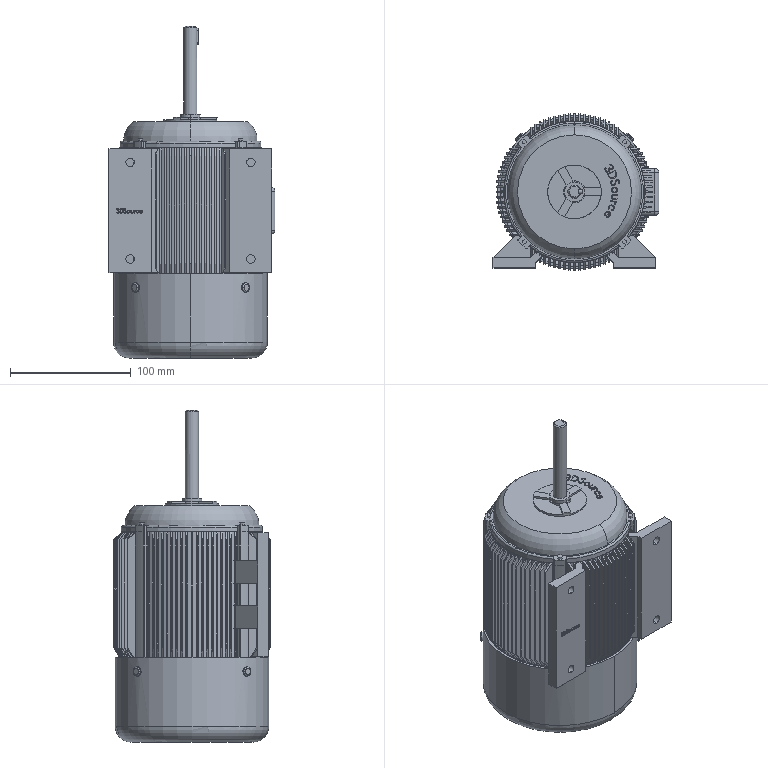Part | NX | features BREP 6, DATUM_CSYS 3, EXTRUDE 3, SKETCH 3, BLEND 2, CHAMFER 1 | 7 solids | 1163 faces | box 137.5 x 130 x 275 mm | volume 2091891 mm3 | cylinder 499 | plane 486 | cone 155 | torus 19 | sphere 4 | commonest cylinder face diameters 130 x95 117 x85 120.25 x77 2.08 x20 7 x16 123.5 x10